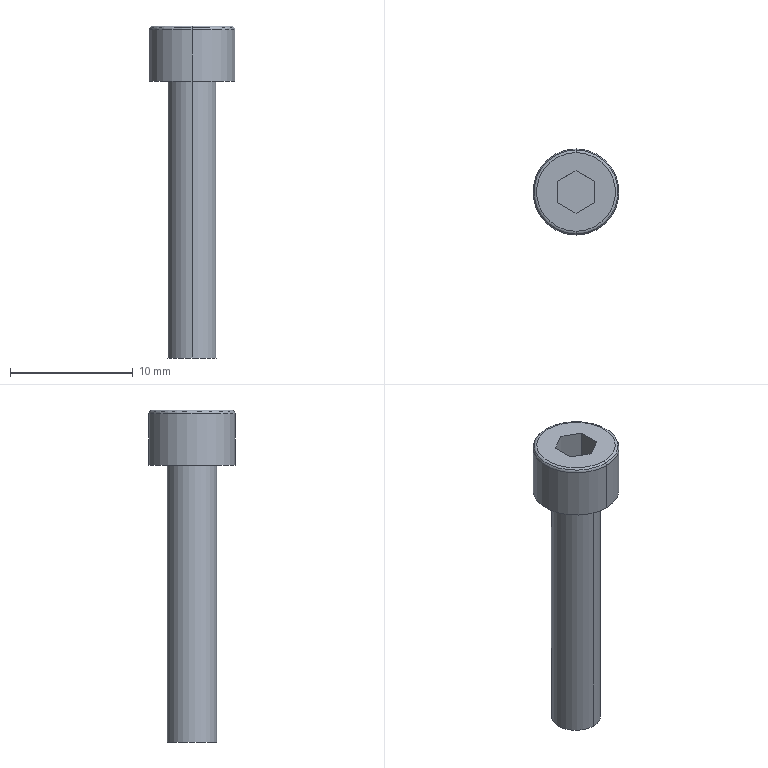Part | Creo | 1 solid | 18 faces | box 7 x 7 x 27 mm | volume 436.801 mm3 | plane 10 | cylinder 4 | torus 4 | commonest cylinder face diameters 4 x2 7 x2
STEP:
#1=CARTESIAN_POINT('',(-184.,117.995,-80.591));
#2=VERTEX_POINT('',#1);
#3=CARTESIAN_POINT('',(-184.,121.995,-80.591));
#4=VERTEX_POINT('',#3);
#5=CARTESIAN_POINT('',(-184.,119.995,-80.591));
#6=DIRECTION('',(0.,0.,-1.));
#7=DIRECTION('',(0.,-1.,0.));
#8=AXIS2_PLACEMENT_3D('',#5,#6,#7);
#9=CIRCLE('',#8,2.);
#10=EDGE_CURVE('',#2,#4,#9,.T.);
#11=ORIENTED_EDGE('',*,*,#10,.F.);
#12=CARTESIAN_POINT('',(-184.,119.995,-80.591));
#13=DIRECTION('',(0.,0.,-1.));
#14=DIRECTION('',(0.,1.,0.));
#15=AXIS2_PLACEMENT_3D('',#12,#13,#14);
#16=CIRCLE('',#15,2.);
#17=EDGE_CURVE('',#4,#2,#16,.T.);
#18=ORIENTED_EDGE('',*,*,#17,.F.);
#19=EDGE_LOOP('',(#11,#18));
#20=FACE_OUTER_BOUND('',#19,.F.);
#21=CARTESIAN_POINT('',(-184.,119.995,-80.591));
#22=DIRECTION('',(0.,0.,-1.));
#23=DIRECTION('',(0.,-1.,0.));
#24=AXIS2_PLACEMENT_3D('',#21,#22,#23);
#25=PLANE('',#24);
#26=ADVANCED_FACE('',(#20),#25,.T.);
#27=CARTESIAN_POINT('',(-184.,121.995,-58.091));
#28=VERTEX_POINT('',#27);
#29=CARTESIAN_POINT('',(-184.,117.995,-58.091));
#30=VERTEX_POINT('',#29);
#31=CARTESIAN_POINT('',(-184.,119.995,-58.091));
#32=DIRECTION('',(0.,0.,1.));
#33=DIRECTION('',(0.,1.,0.));
#34=AXIS2_PLACEMENT_3D('',#31,#32,#33);
#35=CIRCLE('',#34,2.);
#36=EDGE_CURVE('',#28,#30,#35,.T.);
#37=ORIENTED_EDGE('',*,*,#36,.T.);
#38=CARTESIAN_POINT('',(-184.,117.995,-58.091));
#39=DIRECTION('',(0.,0.,-1.));
#40=VECTOR('',#39,22.5);
#41=LINE('',#38,#40);
#42=EDGE_CURVE('',#30,#2,#41,.T.);
#43=ORIENTED_EDGE('',*,*,#42,.T.);
#44=ORIENTED_EDGE('',*,*,#10,.T.);
#45=CARTESIAN_POINT('',(-184.,121.995,-58.091));
#46=DIRECTION('',(0.,0.,-1.));
#47=VECTOR('',#46,22.5);
#48=LINE('',#45,#47);
#49=EDGE_CURVE('',#28,#4,#48,.T.);
#50=ORIENTED_EDGE('',*,*,#49,.F.);
#51=EDGE_LOOP('',(#37,#43,#44,#50));
#52=FACE_OUTER_BOUND('',#51,.F.);
#53=CARTESIAN_POINT('',(-184.,119.995,-53.591));
#54=DIRECTION('',(0.,0.,-1.));
#55=DIRECTION('',(0.,-1.,0.));
#56=AXIS2_PLACEMENT_3D('',#53,#54,#55);
#57=CYLINDRICAL_SURFACE('',#56,2.);
#58=ADVANCED_FACE('',(#52),#57,.T.);
#59=CARTESIAN_POINT('',(-184.,116.495,-58.091));
#60=VERTEX_POINT('',#59);
#61=CARTESIAN_POINT('',(-184.,123.495,-58.091));
#62=VERTEX_POINT('',#61);
#63=CARTESIAN_POINT('',(-184.,119.995,-58.091));
#64=DIRECTION('',(0.,0.,-1.));
#65=DIRECTION('',(0.,-1.,0.));
#66=AXIS2_PLACEMENT_3D('',#63,#64,#65);
#67=CIRCLE('',#66,3.5);
#68=EDGE_CURVE('',#60,#62,#67,.T.);
#69=ORIENTED_EDGE('',*,*,#68,.F.);
#70=CARTESIAN_POINT('',(-184.,119.995,-58.091));
#71=DIRECTION('',(0.,0.,-1.));
#72=DIRECTION('',(0.,1.,0.));
#73=AXIS2_PLACEMENT_3D('',#70,#71,#72);
#74=CIRCLE('',#73,3.5);
#75=EDGE_CURVE('',#62,#60,#74,.T.);
#76=ORIENTED_EDGE('',*,*,#75,.F.);
#77=EDGE_LOOP('',(#69,#76));
#78=FACE_OUTER_BOUND('',#77,.F.);
#79=CARTESIAN_POINT('',(-184.,119.995,-58.091));
#80=DIRECTION('',(0.,0.,1.));
#81=DIRECTION('',(0.,-1.,0.));
#82=AXIS2_PLACEMENT_3D('',#79,#80,#81);
#83=CIRCLE('',#82,2.);
#84=EDGE_CURVE('',#30,#28,#83,.T.);
#85=ORIENTED_EDGE('',*,*,#84,.F.);
#86=ORIENTED_EDGE('',*,*,#36,.F.);
#87=EDGE_LOOP('',(#85,#86));
#88=FACE_BOUND('',#87,.F.);
#89=CARTESIAN_POINT('',(-186.,119.995,-58.091));
#90=DIRECTION('',(0.,0.,-1.));
#91=DIRECTION('',(0.,-1.,0.));
#92=AXIS2_PLACEMENT_3D('',#89,#90,#91);
#93=PLANE('',#92);
#94=ADVANCED_FACE('',(#78,#88),#93,.T.);
#95=CARTESIAN_POINT('',(-184.,123.495,-53.891));
#96=VERTEX_POINT('',#95);
#97=CARTESIAN_POINT('',(-184.,116.495,-53.891));
#98=VERTEX_POINT('',#97);
#99=CARTESIAN_POINT('',(-184.,119.995,-53.891));
#100=DIRECTION('',(0.,0.,1.));
#101=DIRECTION('',(0.,1.,0.));
#102=AXIS2_PLACEMENT_3D('',#99,#100,#101);
#103=CIRCLE('',#102,3.5);
#104=EDGE_CURVE('',#96,#98,#103,.T.);
#105=ORIENTED_EDGE('',*,*,#104,.T.);
#106=CARTESIAN_POINT('',(-184.,116.495,-53.891));
#107=DIRECTION('',(0.,0.,-1.));
#108=VECTOR('',#107,4.2);
#109=LINE('',#106,#108);
#110=EDGE_CURVE('',#98,#60,#109,.T.);
#111=ORIENTED_EDGE('',*,*,#110,.T.);
#112=ORIENTED_EDGE('',*,*,#68,.T.);
#113=CARTESIAN_POINT('',(-184.,123.495,-53.891));
#114=DIRECTION('',(0.,0.,-1.));
#115=VECTOR('',#114,4.2);
#116=LINE('',#113,#115);
#117=EDGE_CURVE('',#96,#62,#116,.T.);
#118=ORIENTED_EDGE('',*,*,#117,.F.);
#119=EDGE_LOOP('',(#105,#111,#112,#118));
#120=FACE_OUTER_BOUND('',#119,.F.);
#121=CARTESIAN_POINT('',(-184.,119.995,-53.591));
#122=DIRECTION('',(0.,0.,-1.));
#123=DIRECTION('',(0.,-1.,0.));
#124=AXIS2_PLACEMENT_3D('',#121,#122,#123);
#125=CYLINDRICAL_SURFACE('',#124,3.5);
#126=ADVANCED_FACE('',(#120),#125,.T.);
#127=ORIENTED_EDGE('',*,*,#104,.F.);
#128=CARTESIAN_POINT('',(-184.,123.407,-53.679));
#129=VERTEX_POINT('',#128);
#130=CARTESIAN_POINT('',(-184.,123.195,-53.891));
#131=DIRECTION('',(1.,0.,0.));
#132=DIRECTION('',(0.,1.,0.));
#133=AXIS2_PLACEMENT_3D('',#130,#131,#132);
#134=CIRCLE('',#133,0.3);
#135=EDGE_CURVE('',#96,#129,#134,.T.);
#136=ORIENTED_EDGE('',*,*,#135,.T.);
#137=CARTESIAN_POINT('',(-184.,116.583,-53.679));
#138=VERTEX_POINT('',#137);
#139=CARTESIAN_POINT('',(-184.,119.995,-53.679));
#140=DIRECTION('',(0.,0.,1.));
#141=DIRECTION('',(0.,1.,0.));
#142=AXIS2_PLACEMENT_3D('',#139,#140,#141);
#143=CIRCLE('',#142,3.412);
#144=EDGE_CURVE('',#129,#138,#143,.T.);
#145=ORIENTED_EDGE('',*,*,#144,.T.);
#146=CARTESIAN_POINT('',(-184.,116.795,-53.891));
#147=DIRECTION('',(-1.,0.,0.));
#148=DIRECTION('',(0.,-1.,0.));
#149=AXIS2_PLACEMENT_3D('',#146,#147,#148);
#150=CIRCLE('',#149,0.3);
#151=EDGE_CURVE('',#98,#138,#150,.T.);
#152=ORIENTED_EDGE('',*,*,#151,.F.);
#153=EDGE_LOOP('',(#127,#136,#145,#152));
#154=FACE_OUTER_BOUND('',#153,.F.);
#155=CARTESIAN_POINT('',(-184.,119.995,-53.891));
#156=DIRECTION('',(0.,0.,1.));
#157=DIRECTION('',(0.,1.,0.));
#158=AXIS2_PLACEMENT_3D('',#155,#156,#157);
#159=TOROIDAL_SURFACE('',#158,3.2,0.3);
#160=ADVANCED_FACE('',(#154),#159,.T.);
#161=CARTESIAN_POINT('',(-184.,119.995,-53.891));
#162=DIRECTION('',(0.,0.,1.));
#163=DIRECTION('',(0.,-1.,0.));
#164=AXIS2_PLACEMENT_3D('',#161,#162,#163);
#165=CIRCLE('',#164,3.5);
#166=EDGE_CURVE('',#98,#96,#165,.T.);
#167=ORIENTED_EDGE('',*,*,#166,.F.);
#168=ORIENTED_EDGE('',*,*,#151,.T.);
#169=CARTESIAN_POINT('',(-184.,119.995,-53.679));
#170=DIRECTION('',(0.,0.,1.));
#171=DIRECTION('',(0.,-1.,0.));
#172=AXIS2_PLACEMENT_3D('',#169,#170,#171);
#173=CIRCLE('',#172,3.412);
#174=EDGE_CURVE('',#138,#129,#173,.T.);
#175=ORIENTED_EDGE('',*,*,#174,.T.);
#176=ORIENTED_EDGE('',*,*,#135,.F.);
#177=EDGE_LOOP('',(#167,#168,#175,#176));
#178=FACE_OUTER_BOUND('',#177,.F.);
#179=CARTESIAN_POINT('',(-184.,119.995,-53.891));
#180=DIRECTION('',(0.,0.,1.));
#181=DIRECTION('',(0.,1.,0.));
#182=AXIS2_PLACEMENT_3D('',#179,#180,#181);
#183=TOROIDAL_SURFACE('',#182,3.2,0.3);
#184=ADVANCED_FACE('',(#178),#183,.T.);
#185=ORIENTED_EDGE('',*,*,#166,.T.);
#186=ORIENTED_EDGE('',*,*,#117,.T.);
#187=ORIENTED_EDGE('',*,*,#75,.T.);
#188=ORIENTED_EDGE('',*,*,#110,.F.);
#189=EDGE_LOOP('',(#185,#186,#187,#188));
#190=FACE_OUTER_BOUND('',#189,.F.);
#191=CARTESIAN_POINT('',(-184.,119.995,-53.591));
#192=DIRECTION('',(0.,0.,-1.));
#193=DIRECTION('',(0.,-1.,0.));
#194=AXIS2_PLACEMENT_3D('',#191,#192,#193);
#195=CYLINDRICAL_SURFACE('',#194,3.5);
#196=ADVANCED_FACE('',(#190),#195,.T.);
#197=CARTESIAN_POINT('',(-184.,116.795,-53.591));
#198=VERTEX_POINT('',#197);
#199=CARTESIAN_POINT('',(-184.,123.195,-53.591));
#200=VERTEX_POINT('',#199);
#201=CARTESIAN_POINT('',(-184.,119.995,-53.591));
#202=DIRECTION('',(0.,0.,1.));
#203=DIRECTION('',(0.,-1.,0.));
#204=AXIS2_PLACEMENT_3D('',#201,#202,#203);
#205=CIRCLE('',#204,3.2);
#206=EDGE_CURVE('',#198,#200,#205,.T.);
#207=ORIENTED_EDGE('',*,*,#206,.T.);
#208=CARTESIAN_POINT('',(-184.,123.195,-53.891));
#209=DIRECTION('',(1.,0.,0.));
#210=DIRECTION('',(0.,0.7071,0.7071));
#211=AXIS2_PLACEMENT_3D('',#208,#209,#210);
#212=CIRCLE('',#211,0.3);
#213=EDGE_CURVE('',#129,#200,#212,.T.);
#214=ORIENTED_EDGE('',*,*,#213,.F.);
#215=ORIENTED_EDGE('',*,*,#174,.F.);
#216=CARTESIAN_POINT('',(-184.,116.795,-53.891));
#217=DIRECTION('',(-1.,0.,0.));
#218=DIRECTION('',(0.,-0.7071,0.7071));
#219=AXIS2_PLACEMENT_3D('',#216,#217,#218);
#220=CIRCLE('',#219,0.3);
#221=EDGE_CURVE('',#138,#198,#220,.T.);
#222=ORIENTED_EDGE('',*,*,#221,.T.);
#223=EDGE_LOOP('',(#207,#214,#215,#222));
#224=FACE_OUTER_BOUND('',#223,.F.);
#225=CARTESIAN_POINT('',(-184.,119.995,-53.891));
#226=DIRECTION('',(0.,0.,1.));
#227=DIRECTION('',(0.,1.,0.));
#228=AXIS2_PLACEMENT_3D('',#225,#226,#227);
#229=TOROIDAL_SURFACE('',#228,3.2,0.3);
#230=ADVANCED_FACE('',(#224),#229,.T.);
#231=CARTESIAN_POINT('',(-184.,119.995,-53.591));
#232=DIRECTION('',(0.,0.,1.));
#233=DIRECTION('',(0.,1.,0.));
#234=AXIS2_PLACEMENT_3D('',#231,#232,#233);
#235=CIRCLE('',#234,3.2);
#236=EDGE_CURVE('',#200,#198,#235,.T.);
#237=ORIENTED_EDGE('',*,*,#236,.F.);
#238=ORIENTED_EDGE('',*,*,#206,.F.);
#239=EDGE_LOOP('',(#237,#238));
#240=FACE_OUTER_BOUND('',#239,.F.);
#241=CARTESIAN_POINT('',(-182.5,119.129,-53.591));
#242=VERTEX_POINT('',#241);
#243=CARTESIAN_POINT('',(-184.,118.263,-53.591));
#244=VERTEX_POINT('',#243);
#245=CARTESIAN_POINT('',(-182.5,119.129,-53.591));
#246=DIRECTION('',(-0.866,-0.5,0.));
#247=VECTOR('',#246,1.732);
#248=LINE('',#245,#247);
#249=EDGE_CURVE('',#242,#244,#248,.T.);
#250=ORIENTED_EDGE('',*,*,#249,.F.);
#251=CARTESIAN_POINT('',(-182.5,120.861,-53.591));
#252=VERTEX_POINT('',#251);
#253=CARTESIAN_POINT('',(-182.5,120.861,-53.591));
#254=DIRECTION('',(0.,-1.,0.));
#255=VECTOR('',#254,1.732);
#256=LINE('',#253,#255);
#257=EDGE_CURVE('',#252,#242,#256,.T.);
#258=ORIENTED_EDGE('',*,*,#257,.F.);
#259=CARTESIAN_POINT('',(-184.,121.727,-53.591));
#260=VERTEX_POINT('',#259);
#261=CARTESIAN_POINT('',(-184.,121.727,-53.591));
#262=DIRECTION('',(0.866,-0.5,0.));
#263=VECTOR('',#262,1.732);
#264=LINE('',#261,#263);
#265=EDGE_CURVE('',#260,#252,#264,.T.);
#266=ORIENTED_EDGE('',*,*,#265,.F.);
#267=CARTESIAN_POINT('',(-185.5,120.861,-53.591));
#268=VERTEX_POINT('',#267);
#269=CARTESIAN_POINT('',(-185.5,120.861,-53.591));
#270=DIRECTION('',(0.866,0.5,0.));
#271=VECTOR('',#270,1.732);
#272=LINE('',#269,#271);
#273=EDGE_CURVE('',#268,#260,#272,.T.);
#274=ORIENTED_EDGE('',*,*,#273,.F.);
#275=CARTESIAN_POINT('',(-185.5,119.129,-53.591));
#276=VERTEX_POINT('',#275);
#277=CARTESIAN_POINT('',(-185.5,119.129,-53.591));
#278=DIRECTION('',(0.,1.,0.));
#279=VECTOR('',#278,1.732);
#280=LINE('',#277,#279);
#281=EDGE_CURVE('',#276,#268,#280,.T.);
#282=ORIENTED_EDGE('',*,*,#281,.F.);
#283=CARTESIAN_POINT('',(-184.,118.263,-53.591));
#284=DIRECTION('',(-0.866,0.5,0.));
#285=VECTOR('',#284,1.732);
#286=LINE('',#283,#285);
#287=EDGE_CURVE('',#244,#276,#286,.T.);
#288=ORIENTED_EDGE('',*,*,#287,.F.);
#289=EDGE_LOOP('',(#250,#258,#266,#274,#282,#288));
#290=FACE_BOUND('',#289,.F.);
#291=CARTESIAN_POINT('',(-187.5,119.995,-53.591));
#292=DIRECTION('',(0.,0.,1.));
#293=DIRECTION('',(0.,1.,0.));
#294=AXIS2_PLACEMENT_3D('',#291,#292,#293);
#295=PLANE('',#294);
#296=ADVANCED_FACE('',(#240,#290),#295,.T.);
#297=ORIENTED_EDGE('',*,*,#236,.T.);
#298=ORIENTED_EDGE('',*,*,#221,.F.);
#299=ORIENTED_EDGE('',*,*,#144,.F.);
#300=ORIENTED_EDGE('',*,*,#213,.T.);
#301=EDGE_LOOP('',(#297,#298,#299,#300));
#302=FACE_OUTER_BOUND('',#301,.F.);
#303=CARTESIAN_POINT('',(-184.,119.995,-53.891));
#304=DIRECTION('',(0.,0.,1.));
#305=DIRECTION('',(0.,1.,0.));
#306=AXIS2_PLACEMENT_3D('',#303,#304,#305);
#307=TOROIDAL_SURFACE('',#306,3.2,0.3);
#308=ADVANCED_FACE('',(#302),#307,.T.);
#309=ORIENTED_EDGE('',*,*,#249,.T.);
#310=CARTESIAN_POINT('',(-184.,118.263,-55.991));
#311=VERTEX_POINT('',#310);
#312=CARTESIAN_POINT('',(-184.,118.263,-55.991));
#313=DIRECTION('',(0.,0.,1.));
#314=VECTOR('',#313,2.4);
#315=LINE('',#312,#314);
#316=EDGE_CURVE('',#311,#244,#315,.T.);
#317=ORIENTED_EDGE('',*,*,#316,.F.);
#318=CARTESIAN_POINT('',(-182.5,119.129,-55.991));
#319=VERTEX_POINT('',#318);
#320=CARTESIAN_POINT('',(-184.,118.263,-55.991));
#321=DIRECTION('',(0.866,0.5,0.));
#322=VECTOR('',#321,1.732);
#323=LINE('',#320,#322);
#324=EDGE_CURVE('',#311,#319,#323,.T.);
#325=ORIENTED_EDGE('',*,*,#324,.T.);
#326=CARTESIAN_POINT('',(-182.5,119.129,-55.991));
#327=DIRECTION('',(0.,0.,1.));
#328=VECTOR('',#327,2.4);
#329=LINE('',#326,#328);
#330=EDGE_CURVE('',#319,#242,#329,.T.);
#331=ORIENTED_EDGE('',*,*,#330,.T.);
#332=EDGE_LOOP('',(#309,#317,#325,#331));
#333=FACE_OUTER_BOUND('',#332,.F.);
#334=CARTESIAN_POINT('',(-184.,118.263,-55.991));
#335=DIRECTION('',(0.5,-0.866,0.));
#336=DIRECTION('',(0.866,0.5,0.));
#337=AXIS2_PLACEMENT_3D('',#334,#335,#336);
#338=PLANE('',#337);
#339=ADVANCED_FACE('',(#333),#338,.F.);
#340=ORIENTED_EDGE('',*,*,#287,.T.);
#341=CARTESIAN_POINT('',(-185.5,119.129,-55.991));
#342=VERTEX_POINT('',#341);
#343=CARTESIAN_POINT('',(-185.5,119.129,-55.991));
#344=DIRECTION('',(0.,0.,1.));
#345=VECTOR('',#344,2.4);
#346=LINE('',#343,#345);
#347=EDGE_CURVE('',#342,#276,#346,.T.);
#348=ORIENTED_EDGE('',*,*,#347,.F.);
#349=CARTESIAN_POINT('',(-185.5,119.129,-55.991));
#350=DIRECTION('',(0.866,-0.5,0.));
#351=VECTOR('',#350,1.732);
#352=LINE('',#349,#351);
#353=EDGE_CURVE('',#342,#311,#352,.T.);
#354=ORIENTED_EDGE('',*,*,#353,.T.);
#355=ORIENTED_EDGE('',*,*,#316,.T.);
#356=EDGE_LOOP('',(#340,#348,#354,#355));
#357=FACE_OUTER_BOUND('',#356,.F.);
#358=CARTESIAN_POINT('',(-185.5,119.129,-55.991));
#359=DIRECTION('',(-0.5,-0.866,0.));
#360=DIRECTION('',(0.866,-0.5,0.));
#361=AXIS2_PLACEMENT_3D('',#358,#359,#360);
#362=PLANE('',#361);
#363=ADVANCED_FACE('',(#357),#362,.F.);
#364=ORIENTED_EDGE('',*,*,#281,.T.);
#365=CARTESIAN_POINT('',(-185.5,120.861,-55.991));
#366=VERTEX_POINT('',#365);
#367=CARTESIAN_POINT('',(-185.5,120.861,-55.991));
#368=DIRECTION('',(0.,0.,1.));
#369=VECTOR('',#368,2.4);
#370=LINE('',#367,#369);
#371=EDGE_CURVE('',#366,#268,#370,.T.);
#372=ORIENTED_EDGE('',*,*,#371,.F.);
#373=CARTESIAN_POINT('',(-185.5,120.861,-55.991));
#374=DIRECTION('',(0.,-1.,0.));
#375=VECTOR('',#374,1.732);
#376=LINE('',#373,#375);
#377=EDGE_CURVE('',#366,#342,#376,.T.);
#378=ORIENTED_EDGE('',*,*,#377,.T.);
#379=ORIENTED_EDGE('',*,*,#347,.T.);
#380=EDGE_LOOP('',(#364,#372,#378,#379));
#381=FACE_OUTER_BOUND('',#380,.F.);
#382=CARTESIAN_POINT('',(-185.5,120.861,-55.991));
#383=DIRECTION('',(-1.,0.,0.));
#384=DIRECTION('',(0.,-1.,0.));
#385=AXIS2_PLACEMENT_3D('',#382,#383,#384);
#386=PLANE('',#385);
#387=ADVANCED_FACE('',(#381),#386,.F.);
#388=ORIENTED_EDGE('',*,*,#273,.T.);
#389=CARTESIAN_POINT('',(-184.,121.727,-55.991));
#390=VERTEX_POINT('',#389);
#391=CARTESIAN_POINT('',(-184.,121.727,-55.991));
#392=DIRECTION('',(0.,0.,1.));
#393=VECTOR('',#392,2.4);
#394=LINE('',#391,#393);
#395=EDGE_CURVE('',#390,#260,#394,.T.);
#396=ORIENTED_EDGE('',*,*,#395,.F.);
#397=CARTESIAN_POINT('',(-184.,121.727,-55.991));
#398=DIRECTION('',(-0.866,-0.5,0.));
#399=VECTOR('',#398,1.732);
#400=LINE('',#397,#399);
#401=EDGE_CURVE('',#390,#366,#400,.T.);
#402=ORIENTED_EDGE('',*,*,#401,.T.);
#403=ORIENTED_EDGE('',*,*,#371,.T.);
#404=EDGE_LOOP('',(#388,#396,#402,#403));
#405=FACE_OUTER_BOUND('',#404,.F.);
#406=CARTESIAN_POINT('',(-184.,121.727,-55.991));
#407=DIRECTION('',(-0.5,0.866,0.));
#408=DIRECTION('',(-0.866,-0.5,0.));
#409=AXIS2_PLACEMENT_3D('',#406,#407,#408);
#410=PLANE('',#409);
#411=ADVANCED_FACE('',(#405),#410,.F.);
#412=ORIENTED_EDGE('',*,*,#265,.T.);
#413=CARTESIAN_POINT('',(-182.5,120.861,-55.991));
#414=VERTEX_POINT('',#413);
#415=CARTESIAN_POINT('',(-182.5,120.861,-55.991));
#416=DIRECTION('',(0.,0.,1.));
#417=VECTOR('',#416,2.4);
#418=LINE('',#415,#417);
#419=EDGE_CURVE('',#414,#252,#418,.T.);
#420=ORIENTED_EDGE('',*,*,#419,.F.);
#421=CARTESIAN_POINT('',(-182.5,120.861,-55.991));
#422=DIRECTION('',(-0.866,0.5,0.));
#423=VECTOR('',#422,1.732);
#424=LINE('',#421,#423);
#425=EDGE_CURVE('',#414,#390,#424,.T.);
#426=ORIENTED_EDGE('',*,*,#425,.T.);
#427=ORIENTED_EDGE('',*,*,#395,.T.);
#428=EDGE_LOOP('',(#412,#420,#426,#427));
#429=FACE_OUTER_BOUND('',#428,.F.);
#430=CARTESIAN_POINT('',(-182.5,120.861,-55.991));
#431=DIRECTION('',(0.5,0.866,0.));
#432=DIRECTION('',(-0.866,0.5,0.));
#433=AXIS2_PLACEMENT_3D('',#430,#431,#432);
#434=PLANE('',#433);
#435=ADVANCED_FACE('',(#429),#434,.F.);
#436=ORIENTED_EDGE('',*,*,#257,.T.);
#437=ORIENTED_EDGE('',*,*,#330,.F.);
#438=CARTESIAN_POINT('',(-182.5,119.129,-55.991));
#439=DIRECTION('',(0.,1.,0.));
#440=VECTOR('',#439,1.732);
#441=LINE('',#438,#440);
#442=EDGE_CURVE('',#319,#414,#441,.T.);
#443=ORIENTED_EDGE('',*,*,#442,.T.);
#444=ORIENTED_EDGE('',*,*,#419,.T.);
#445=EDGE_LOOP('',(#436,#437,#443,#444));
#446=FACE_OUTER_BOUND('',#445,.F.);
#447=CARTESIAN_POINT('',(-182.5,119.129,-55.991));
#448=DIRECTION('',(1.,0.,0.));
#449=DIRECTION('',(0.,1.,0.));
#450=AXIS2_PLACEMENT_3D('',#447,#448,#449);
#451=PLANE('',#450);
#452=ADVANCED_FACE('',(#446),#451,.F.);
#453=ORIENTED_EDGE('',*,*,#324,.F.);
#454=ORIENTED_EDGE('',*,*,#353,.F.);
#455=ORIENTED_EDGE('',*,*,#377,.F.);
#456=ORIENTED_EDGE('',*,*,#401,.F.);
#457=ORIENTED_EDGE('',*,*,#425,.F.);
#458=ORIENTED_EDGE('',*,*,#442,.F.);
#459=EDGE_LOOP('',(#453,#454,#455,#456,#457,#458));
#460=FACE_OUTER_BOUND('',#459,.F.);
#461=CARTESIAN_POINT('',(-190.,119.995,-55.991));
#462=DIRECTION('',(0.,0.,1.));
#463=DIRECTION('',(0.,1.,0.));
#464=AXIS2_PLACEMENT_3D('',#461,#462,#463);
#465=PLANE('',#464);
#466=ADVANCED_FACE('',(#460),#465,.T.);
#467=ORIENTED_EDGE('',*,*,#84,.T.);
#468=ORIENTED_EDGE('',*,*,#49,.T.);
#469=ORIENTED_EDGE('',*,*,#17,.T.);
#470=ORIENTED_EDGE('',*,*,#42,.F.);
#471=EDGE_LOOP('',(#467,#468,#469,#470));
#472=FACE_OUTER_BOUND('',#471,.F.);
#473=CARTESIAN_POINT('',(-184.,119.995,-53.591));
#474=DIRECTION('',(0.,0.,-1.));
#475=DIRECTION('',(0.,-1.,0.));
#476=AXIS2_PLACEMENT_3D('',#473,#474,#475);
#477=CYLINDRICAL_SURFACE('',#476,2.);
#478=ADVANCED_FACE('',(#472),#477,.T.);
#479=CLOSED_SHELL('',(#26,#58,#94,#126,#160,#184,#196,#230,#296,#308,#339,#363,#387,#411,#435,#452,#466,#478));
#480=MANIFOLD_SOLID_BREP('',#479);
#481=(LENGTH_UNIT()NAMED_UNIT(*)SI_UNIT(.MILLI.,.METRE.));
#482=UNCERTAINTY_MEASURE_WITH_UNIT(LENGTH_MEASURE(0.002876),#481,'','');
#483=(NAMED_UNIT(*)PLANE_ANGLE_UNIT()SI_UNIT($,.RADIAN.));
#484=PLANE_ANGLE_MEASURE_WITH_UNIT(PLANE_ANGLE_MEASURE(0.01745),#483);
#485=(CONVERSION_BASED_UNIT('DEGREE',#484)NAMED_UNIT(*)PLANE_ANGLE_UNIT());
#486=(NAMED_UNIT(*)SI_UNIT($,.STERADIAN.)SOLID_ANGLE_UNIT());
#487=(GEOMETRIC_REPRESENTATION_CONTEXT(3)GLOBAL_UNCERTAINTY_ASSIGNED_CONTEXT((#482))GLOBAL_UNIT_ASSIGNED_CONTEXT((#481,#485,#486))REPRESENTATION_CONTEXT('',''));
#488=ADVANCED_BREP_SHAPE_REPRESENTATION('',(#480),#487);